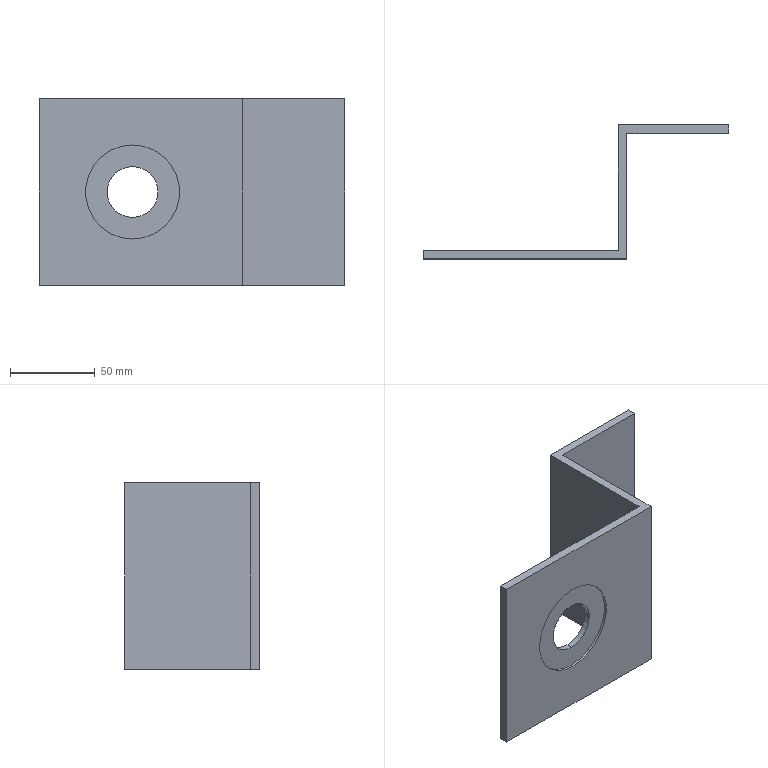Part | STEP file | Guide wheel mechanism revised.sldasm-Part-360 | 1 solid | 15 faces | box 180 x 79 x 110 mm | volume 133597 mm3 | plane 11 | cylinder 4 | commonest cylinder face diameters 30 x2 55.5 x2
STEP:
#1=CARTESIAN_POINT('',(55.,5.,15.));
#2=VERTEX_POINT('',#1);
#3=CARTESIAN_POINT('',(55.,5.,-15.));
#4=VERTEX_POINT('',#3);
#5=CARTESIAN_POINT('',(55.,5.,0.));
#6=DIRECTION('',(0.,-1.,0.));
#7=DIRECTION('',(0.,0.,1.));
#8=AXIS2_PLACEMENT_3D('',#5,#6,#7);
#9=CIRCLE('',#8,15.);
#10=EDGE_CURVE('',#2,#4,#9,.T.);
#11=ORIENTED_EDGE('',*,*,#10,.F.);
#12=CARTESIAN_POINT('',(55.,1.5,15.));
#13=VERTEX_POINT('',#12);
#14=CARTESIAN_POINT('',(55.,79.001,15.));
#15=DIRECTION('',(0.,-1.,0.));
#16=VECTOR('',#15,1000.);
#17=LINE('',#14,#16);
#18=EDGE_CURVE('',#2,#13,#17,.T.);
#19=ORIENTED_EDGE('',*,*,#18,.T.);
#20=CARTESIAN_POINT('',(55.,1.5,-15.));
#21=VERTEX_POINT('',#20);
#22=CARTESIAN_POINT('',(55.,1.5,0.));
#23=DIRECTION('',(0.,-1.,0.));
#24=DIRECTION('',(0.,0.,-1.));
#25=AXIS2_PLACEMENT_3D('',#22,#23,#24);
#26=CIRCLE('',#25,15.);
#27=EDGE_CURVE('',#13,#21,#26,.T.);
#28=ORIENTED_EDGE('',*,*,#27,.T.);
#29=CARTESIAN_POINT('',(55.,79.001,-15.));
#30=DIRECTION('',(0.,-1.,0.));
#31=VECTOR('',#30,1000.);
#32=LINE('',#29,#31);
#33=EDGE_CURVE('',#4,#21,#32,.T.);
#34=ORIENTED_EDGE('',*,*,#33,.F.);
#35=EDGE_LOOP('',(#11,#19,#28,#34));
#36=FACE_OUTER_BOUND('',#35,.T.);
#37=CARTESIAN_POINT('',(55.,79.001,0.));
#38=DIRECTION('',(0.,-1.,0.));
#39=DIRECTION('',(0.,0.,-1.));
#40=AXIS2_PLACEMENT_3D('',#37,#38,#39);
#41=CYLINDRICAL_SURFACE('',#40,15.);
#42=ADVANCED_FACE('',(#36),#41,.F.);
#43=CARTESIAN_POINT('',(55.,1.5,27.75));
#44=VERTEX_POINT('',#43);
#45=CARTESIAN_POINT('',(55.,1.5,-27.75));
#46=VERTEX_POINT('',#45);
#47=CARTESIAN_POINT('',(55.,1.5,0.));
#48=DIRECTION('',(0.,-1.,0.));
#49=DIRECTION('',(0.,0.,-1.));
#50=AXIS2_PLACEMENT_3D('',#47,#48,#49);
#51=CIRCLE('',#50,27.75);
#52=EDGE_CURVE('',#44,#46,#51,.T.);
#53=ORIENTED_EDGE('',*,*,#52,.F.);
#54=CARTESIAN_POINT('',(55.,0.,27.75));
#55=VERTEX_POINT('',#54);
#56=CARTESIAN_POINT('',(55.,1.5,27.75));
#57=DIRECTION('',(0.,-1.,0.));
#58=VECTOR('',#57,1000.);
#59=LINE('',#56,#58);
#60=EDGE_CURVE('',#44,#55,#59,.T.);
#61=ORIENTED_EDGE('',*,*,#60,.T.);
#62=CARTESIAN_POINT('',(55.,0.,-27.75));
#63=VERTEX_POINT('',#62);
#64=CARTESIAN_POINT('',(55.,0.,0.));
#65=DIRECTION('',(0.,-1.,0.));
#66=DIRECTION('',(0.,0.,-1.));
#67=AXIS2_PLACEMENT_3D('',#64,#65,#66);
#68=CIRCLE('',#67,27.75);
#69=EDGE_CURVE('',#55,#63,#68,.T.);
#70=ORIENTED_EDGE('',*,*,#69,.T.);
#71=CARTESIAN_POINT('',(55.,1.5,-27.75));
#72=DIRECTION('',(0.,-1.,0.));
#73=VECTOR('',#72,1000.);
#74=LINE('',#71,#73);
#75=EDGE_CURVE('',#46,#63,#74,.T.);
#76=ORIENTED_EDGE('',*,*,#75,.F.);
#77=EDGE_LOOP('',(#53,#61,#70,#76));
#78=FACE_OUTER_BOUND('',#77,.T.);
#79=CARTESIAN_POINT('',(55.,1.5,0.));
#80=DIRECTION('',(0.,-1.,0.));
#81=DIRECTION('',(0.,0.,-1.));
#82=AXIS2_PLACEMENT_3D('',#79,#80,#81);
#83=CYLINDRICAL_SURFACE('',#82,27.75);
#84=ADVANCED_FACE('',(#78),#83,.F.);
#85=CARTESIAN_POINT('',(120.,74.,-55.));
#86=VERTEX_POINT('',#85);
#87=CARTESIAN_POINT('',(180.,74.,-55.));
#88=VERTEX_POINT('',#87);
#89=CARTESIAN_POINT('',(120.,74.,-55.));
#90=DIRECTION('',(1.,0.,0.));
#91=VECTOR('',#90,1000.);
#92=LINE('',#89,#91);
#93=EDGE_CURVE('',#86,#88,#92,.T.);
#94=ORIENTED_EDGE('',*,*,#93,.T.);
#95=CARTESIAN_POINT('',(180.,74.,55.));
#96=VERTEX_POINT('',#95);
#97=CARTESIAN_POINT('',(180.,74.,55.));
#98=DIRECTION('',(0.,0.,-1.));
#99=VECTOR('',#98,1000.);
#100=LINE('',#97,#99);
#101=EDGE_CURVE('',#96,#88,#100,.T.);
#102=ORIENTED_EDGE('',*,*,#101,.F.);
#103=CARTESIAN_POINT('',(120.,74.,55.));
#104=VERTEX_POINT('',#103);
#105=CARTESIAN_POINT('',(120.,74.,55.));
#106=DIRECTION('',(1.,0.,0.));
#107=VECTOR('',#106,1000.);
#108=LINE('',#105,#107);
#109=EDGE_CURVE('',#104,#96,#108,.T.);
#110=ORIENTED_EDGE('',*,*,#109,.F.);
#111=CARTESIAN_POINT('',(120.,74.,55.));
#112=DIRECTION('',(0.,0.,-1.));
#113=VECTOR('',#112,1000.);
#114=LINE('',#111,#113);
#115=EDGE_CURVE('',#104,#86,#114,.T.);
#116=ORIENTED_EDGE('',*,*,#115,.T.);
#117=EDGE_LOOP('',(#94,#102,#110,#116));
#118=FACE_OUTER_BOUND('',#117,.T.);
#119=CARTESIAN_POINT('',(120.,74.,55.));
#120=DIRECTION('',(0.,1.,0.));
#121=DIRECTION('',(0.,0.,1.));
#122=AXIS2_PLACEMENT_3D('',#119,#120,#121);
#123=PLANE('',#122);
#124=ADVANCED_FACE('',(#118),#123,.F.);
#125=CARTESIAN_POINT('',(180.,79.,-55.));
#126=VERTEX_POINT('',#125);
#127=CARTESIAN_POINT('',(180.,79.,-55.));
#128=DIRECTION('',(0.,-1.,0.));
#129=VECTOR('',#128,1000.);
#130=LINE('',#127,#129);
#131=EDGE_CURVE('',#126,#88,#130,.T.);
#132=ORIENTED_EDGE('',*,*,#131,.F.);
#133=CARTESIAN_POINT('',(180.,79.,55.));
#134=VERTEX_POINT('',#133);
#135=CARTESIAN_POINT('',(180.,79.,55.));
#136=DIRECTION('',(0.,0.,-1.));
#137=VECTOR('',#136,1000.);
#138=LINE('',#135,#137);
#139=EDGE_CURVE('',#134,#126,#138,.T.);
#140=ORIENTED_EDGE('',*,*,#139,.F.);
#141=CARTESIAN_POINT('',(180.,79.,55.));
#142=DIRECTION('',(0.,-1.,0.));
#143=VECTOR('',#142,1000.);
#144=LINE('',#141,#143);
#145=EDGE_CURVE('',#134,#96,#144,.T.);
#146=ORIENTED_EDGE('',*,*,#145,.T.);
#147=ORIENTED_EDGE('',*,*,#101,.T.);
#148=EDGE_LOOP('',(#132,#140,#146,#147));
#149=FACE_OUTER_BOUND('',#148,.T.);
#150=CARTESIAN_POINT('',(180.,79.,55.));
#151=DIRECTION('',(1.,0.,0.));
#152=DIRECTION('',(0.,0.,-1.));
#153=AXIS2_PLACEMENT_3D('',#150,#151,#152);
#154=PLANE('',#153);
#155=ADVANCED_FACE('',(#149),#154,.T.);
#156=CARTESIAN_POINT('',(115.,79.,-55.));
#157=VERTEX_POINT('',#156);
#158=CARTESIAN_POINT('',(120.,79.,-55.));
#159=DIRECTION('',(1.,0.,0.));
#160=VECTOR('',#159,1000.);
#161=LINE('',#158,#160);
#162=EDGE_CURVE('',#157,#126,#161,.T.);
#163=ORIENTED_EDGE('',*,*,#162,.F.);
#164=CARTESIAN_POINT('',(115.,79.,55.));
#165=VERTEX_POINT('',#164);
#166=CARTESIAN_POINT('',(115.,79.,55.));
#167=DIRECTION('',(0.,0.,-1.));
#168=VECTOR('',#167,1000.);
#169=LINE('',#166,#168);
#170=EDGE_CURVE('',#165,#157,#169,.T.);
#171=ORIENTED_EDGE('',*,*,#170,.F.);
#172=CARTESIAN_POINT('',(120.,79.,55.));
#173=DIRECTION('',(1.,0.,0.));
#174=VECTOR('',#173,1000.);
#175=LINE('',#172,#174);
#176=EDGE_CURVE('',#165,#134,#175,.T.);
#177=ORIENTED_EDGE('',*,*,#176,.T.);
#178=ORIENTED_EDGE('',*,*,#139,.T.);
#179=EDGE_LOOP('',(#163,#171,#177,#178));
#180=FACE_OUTER_BOUND('',#179,.T.);
#181=CARTESIAN_POINT('',(120.,79.,55.));
#182=DIRECTION('',(0.,1.,0.));
#183=DIRECTION('',(0.,0.,1.));
#184=AXIS2_PLACEMENT_3D('',#181,#182,#183);
#185=PLANE('',#184);
#186=ADVANCED_FACE('',(#180),#185,.T.);
#187=CARTESIAN_POINT('',(115.,5.,-55.));
#188=VERTEX_POINT('',#187);
#189=CARTESIAN_POINT('',(115.,0.,-55.));
#190=DIRECTION('',(0.,1.,0.));
#191=VECTOR('',#190,1000.);
#192=LINE('',#189,#191);
#193=EDGE_CURVE('',#188,#157,#192,.T.);
#194=ORIENTED_EDGE('',*,*,#193,.F.);
#195=CARTESIAN_POINT('',(115.,5.,55.));
#196=VERTEX_POINT('',#195);
#197=CARTESIAN_POINT('',(115.,5.,55.));
#198=DIRECTION('',(0.,0.,-1.));
#199=VECTOR('',#198,1000.);
#200=LINE('',#197,#199);
#201=EDGE_CURVE('',#196,#188,#200,.T.);
#202=ORIENTED_EDGE('',*,*,#201,.F.);
#203=CARTESIAN_POINT('',(115.,0.,55.));
#204=DIRECTION('',(0.,1.,0.));
#205=VECTOR('',#204,1000.);
#206=LINE('',#203,#205);
#207=EDGE_CURVE('',#196,#165,#206,.T.);
#208=ORIENTED_EDGE('',*,*,#207,.T.);
#209=ORIENTED_EDGE('',*,*,#170,.T.);
#210=EDGE_LOOP('',(#194,#202,#208,#209));
#211=FACE_OUTER_BOUND('',#210,.T.);
#212=CARTESIAN_POINT('',(115.,0.,55.));
#213=DIRECTION('',(-1.,0.,0.));
#214=DIRECTION('',(0.,0.,1.));
#215=AXIS2_PLACEMENT_3D('',#212,#213,#214);
#216=PLANE('',#215);
#217=ADVANCED_FACE('',(#211),#216,.T.);
#218=CARTESIAN_POINT('',(55.,5.,0.));
#219=DIRECTION('',(0.,-1.,0.));
#220=DIRECTION('',(0.,0.,1.));
#221=AXIS2_PLACEMENT_3D('',#218,#219,#220);
#222=CIRCLE('',#221,15.);
#223=EDGE_CURVE('',#4,#2,#222,.T.);
#224=ORIENTED_EDGE('',*,*,#223,.T.);
#225=ORIENTED_EDGE('',*,*,#10,.T.);
#226=EDGE_LOOP('',(#224,#225));
#227=FACE_BOUND('',#226,.T.);
#228=CARTESIAN_POINT('',(0.,5.,-55.));
#229=VERTEX_POINT('',#228);
#230=CARTESIAN_POINT('',(0.,5.,-55.));
#231=DIRECTION('',(1.,0.,0.));
#232=VECTOR('',#231,1000.);
#233=LINE('',#230,#232);
#234=EDGE_CURVE('',#229,#188,#233,.T.);
#235=ORIENTED_EDGE('',*,*,#234,.F.);
#236=CARTESIAN_POINT('',(0.,5.,55.));
#237=VERTEX_POINT('',#236);
#238=CARTESIAN_POINT('',(0.,5.,55.));
#239=DIRECTION('',(0.,0.,-1.));
#240=VECTOR('',#239,1000.);
#241=LINE('',#238,#240);
#242=EDGE_CURVE('',#237,#229,#241,.T.);
#243=ORIENTED_EDGE('',*,*,#242,.F.);
#244=CARTESIAN_POINT('',(0.,5.,55.));
#245=DIRECTION('',(1.,0.,0.));
#246=VECTOR('',#245,1000.);
#247=LINE('',#244,#246);
#248=EDGE_CURVE('',#237,#196,#247,.T.);
#249=ORIENTED_EDGE('',*,*,#248,.T.);
#250=ORIENTED_EDGE('',*,*,#201,.T.);
#251=EDGE_LOOP('',(#235,#243,#249,#250));
#252=FACE_OUTER_BOUND('',#251,.T.);
#253=CARTESIAN_POINT('',(0.,5.,55.));
#254=DIRECTION('',(0.,1.,0.));
#255=DIRECTION('',(0.,0.,1.));
#256=AXIS2_PLACEMENT_3D('',#253,#254,#255);
#257=PLANE('',#256);
#258=ADVANCED_FACE('',(#227,#252),#257,.T.);
#259=CARTESIAN_POINT('',(0.,0.,-55.));
#260=VERTEX_POINT('',#259);
#261=CARTESIAN_POINT('',(0.,0.,-55.));
#262=DIRECTION('',(0.,1.,0.));
#263=VECTOR('',#262,1000.);
#264=LINE('',#261,#263);
#265=EDGE_CURVE('',#260,#229,#264,.T.);
#266=ORIENTED_EDGE('',*,*,#265,.F.);
#267=CARTESIAN_POINT('',(0.,0.,55.));
#268=VERTEX_POINT('',#267);
#269=CARTESIAN_POINT('',(0.,0.,55.));
#270=DIRECTION('',(0.,0.,-1.));
#271=VECTOR('',#270,1000.);
#272=LINE('',#269,#271);
#273=EDGE_CURVE('',#268,#260,#272,.T.);
#274=ORIENTED_EDGE('',*,*,#273,.F.);
#275=CARTESIAN_POINT('',(0.,0.,55.));
#276=DIRECTION('',(0.,1.,0.));
#277=VECTOR('',#276,1000.);
#278=LINE('',#275,#277);
#279=EDGE_CURVE('',#268,#237,#278,.T.);
#280=ORIENTED_EDGE('',*,*,#279,.T.);
#281=ORIENTED_EDGE('',*,*,#242,.T.);
#282=EDGE_LOOP('',(#266,#274,#280,#281));
#283=FACE_OUTER_BOUND('',#282,.T.);
#284=CARTESIAN_POINT('',(0.,0.,55.));
#285=DIRECTION('',(-1.,0.,0.));
#286=DIRECTION('',(0.,0.,1.));
#287=AXIS2_PLACEMENT_3D('',#284,#285,#286);
#288=PLANE('',#287);
#289=ADVANCED_FACE('',(#283),#288,.T.);
#290=CARTESIAN_POINT('',(55.,0.,0.));
#291=DIRECTION('',(0.,-1.,0.));
#292=DIRECTION('',(0.,0.,-1.));
#293=AXIS2_PLACEMENT_3D('',#290,#291,#292);
#294=CIRCLE('',#293,27.75);
#295=EDGE_CURVE('',#63,#55,#294,.T.);
#296=ORIENTED_EDGE('',*,*,#295,.F.);
#297=ORIENTED_EDGE('',*,*,#69,.F.);
#298=EDGE_LOOP('',(#296,#297));
#299=FACE_BOUND('',#298,.T.);
#300=CARTESIAN_POINT('',(120.,0.,-55.));
#301=VERTEX_POINT('',#300);
#302=CARTESIAN_POINT('',(0.,0.,-55.));
#303=DIRECTION('',(1.,0.,0.));
#304=VECTOR('',#303,1000.);
#305=LINE('',#302,#304);
#306=EDGE_CURVE('',#260,#301,#305,.T.);
#307=ORIENTED_EDGE('',*,*,#306,.T.);
#308=CARTESIAN_POINT('',(120.,0.,55.));
#309=VERTEX_POINT('',#308);
#310=CARTESIAN_POINT('',(120.,0.,55.));
#311=DIRECTION('',(0.,0.,-1.));
#312=VECTOR('',#311,1000.);
#313=LINE('',#310,#312);
#314=EDGE_CURVE('',#309,#301,#313,.T.);
#315=ORIENTED_EDGE('',*,*,#314,.F.);
#316=CARTESIAN_POINT('',(0.,0.,55.));
#317=DIRECTION('',(1.,0.,0.));
#318=VECTOR('',#317,1000.);
#319=LINE('',#316,#318);
#320=EDGE_CURVE('',#268,#309,#319,.T.);
#321=ORIENTED_EDGE('',*,*,#320,.F.);
#322=ORIENTED_EDGE('',*,*,#273,.T.);
#323=EDGE_LOOP('',(#307,#315,#321,#322));
#324=FACE_OUTER_BOUND('',#323,.T.);
#325=CARTESIAN_POINT('',(0.,0.,55.));
#326=DIRECTION('',(0.,1.,0.));
#327=DIRECTION('',(0.,0.,1.));
#328=AXIS2_PLACEMENT_3D('',#325,#326,#327);
#329=PLANE('',#328);
#330=ADVANCED_FACE('',(#299,#324),#329,.F.);
#331=CARTESIAN_POINT('',(120.,0.,-55.));
#332=DIRECTION('',(0.,1.,0.));
#333=VECTOR('',#332,1000.);
#334=LINE('',#331,#333);
#335=EDGE_CURVE('',#301,#86,#334,.T.);
#336=ORIENTED_EDGE('',*,*,#335,.T.);
#337=ORIENTED_EDGE('',*,*,#115,.F.);
#338=CARTESIAN_POINT('',(120.,0.,55.));
#339=DIRECTION('',(0.,1.,0.));
#340=VECTOR('',#339,1000.);
#341=LINE('',#338,#340);
#342=EDGE_CURVE('',#309,#104,#341,.T.);
#343=ORIENTED_EDGE('',*,*,#342,.F.);
#344=ORIENTED_EDGE('',*,*,#314,.T.);
#345=EDGE_LOOP('',(#336,#337,#343,#344));
#346=FACE_OUTER_BOUND('',#345,.T.);
#347=CARTESIAN_POINT('',(120.,0.,55.));
#348=DIRECTION('',(-1.,0.,0.));
#349=DIRECTION('',(0.,0.,1.));
#350=AXIS2_PLACEMENT_3D('',#347,#348,#349);
#351=PLANE('',#350);
#352=ADVANCED_FACE('',(#346),#351,.F.);
#353=ORIENTED_EDGE('',*,*,#109,.T.);
#354=ORIENTED_EDGE('',*,*,#145,.F.);
#355=ORIENTED_EDGE('',*,*,#176,.F.);
#356=ORIENTED_EDGE('',*,*,#207,.F.);
#357=ORIENTED_EDGE('',*,*,#248,.F.);
#358=ORIENTED_EDGE('',*,*,#279,.F.);
#359=ORIENTED_EDGE('',*,*,#320,.T.);
#360=ORIENTED_EDGE('',*,*,#342,.T.);
#361=EDGE_LOOP('',(#353,#354,#355,#356,#357,#358,#359,#360));
#362=FACE_OUTER_BOUND('',#361,.T.);
#363=CARTESIAN_POINT('',(0.,0.,55.));
#364=DIRECTION('',(0.,0.,-1.));
#365=DIRECTION('',(-1.,0.,0.));
#366=AXIS2_PLACEMENT_3D('',#363,#364,#365);
#367=PLANE('',#366);
#368=ADVANCED_FACE('',(#362),#367,.F.);
#369=ORIENTED_EDGE('',*,*,#93,.F.);
#370=ORIENTED_EDGE('',*,*,#335,.F.);
#371=ORIENTED_EDGE('',*,*,#306,.F.);
#372=ORIENTED_EDGE('',*,*,#265,.T.);
#373=ORIENTED_EDGE('',*,*,#234,.T.);
#374=ORIENTED_EDGE('',*,*,#193,.T.);
#375=ORIENTED_EDGE('',*,*,#162,.T.);
#376=ORIENTED_EDGE('',*,*,#131,.T.);
#377=EDGE_LOOP('',(#369,#370,#371,#372,#373,#374,#375,#376));
#378=FACE_OUTER_BOUND('',#377,.T.);
#379=CARTESIAN_POINT('',(0.,0.,-55.));
#380=DIRECTION('',(0.,0.,-1.));
#381=DIRECTION('',(-1.,0.,0.));
#382=AXIS2_PLACEMENT_3D('',#379,#380,#381);
#383=PLANE('',#382);
#384=ADVANCED_FACE('',(#378),#383,.T.);
#385=ORIENTED_EDGE('',*,*,#60,.F.);
#386=CARTESIAN_POINT('',(55.,1.5,0.));
#387=DIRECTION('',(0.,-1.,0.));
#388=DIRECTION('',(0.,0.,-1.));
#389=AXIS2_PLACEMENT_3D('',#386,#387,#388);
#390=CIRCLE('',#389,27.75);
#391=EDGE_CURVE('',#46,#44,#390,.T.);
#392=ORIENTED_EDGE('',*,*,#391,.F.);
#393=ORIENTED_EDGE('',*,*,#75,.T.);
#394=ORIENTED_EDGE('',*,*,#295,.T.);
#395=EDGE_LOOP('',(#385,#392,#393,#394));
#396=FACE_OUTER_BOUND('',#395,.T.);
#397=CARTESIAN_POINT('',(55.,1.5,0.));
#398=DIRECTION('',(0.,-1.,0.));
#399=DIRECTION('',(0.,0.,-1.));
#400=AXIS2_PLACEMENT_3D('',#397,#398,#399);
#401=CYLINDRICAL_SURFACE('',#400,27.75);
#402=ADVANCED_FACE('',(#396),#401,.F.);
#403=CARTESIAN_POINT('',(55.,1.5,0.));
#404=DIRECTION('',(0.,-1.,0.));
#405=DIRECTION('',(0.,0.,-1.));
#406=AXIS2_PLACEMENT_3D('',#403,#404,#405);
#407=CIRCLE('',#406,15.);
#408=EDGE_CURVE('',#21,#13,#407,.T.);
#409=ORIENTED_EDGE('',*,*,#408,.F.);
#410=ORIENTED_EDGE('',*,*,#27,.F.);
#411=EDGE_LOOP('',(#409,#410));
#412=FACE_BOUND('',#411,.T.);
#413=ORIENTED_EDGE('',*,*,#391,.T.);
#414=ORIENTED_EDGE('',*,*,#52,.T.);
#415=EDGE_LOOP('',(#413,#414));
#416=FACE_OUTER_BOUND('',#415,.T.);
#417=CARTESIAN_POINT('',(55.,1.5,0.));
#418=DIRECTION('',(0.,-1.,0.));
#419=DIRECTION('',(0.,0.,-1.));
#420=AXIS2_PLACEMENT_3D('',#417,#418,#419);
#421=PLANE('',#420);
#422=ADVANCED_FACE('',(#412,#416),#421,.T.);
#423=ORIENTED_EDGE('',*,*,#18,.F.);
#424=ORIENTED_EDGE('',*,*,#223,.F.);
#425=ORIENTED_EDGE('',*,*,#33,.T.);
#426=ORIENTED_EDGE('',*,*,#408,.T.);
#427=EDGE_LOOP('',(#423,#424,#425,#426));
#428=FACE_OUTER_BOUND('',#427,.T.);
#429=CARTESIAN_POINT('',(55.,79.001,0.));
#430=DIRECTION('',(0.,-1.,0.));
#431=DIRECTION('',(0.,0.,-1.));
#432=AXIS2_PLACEMENT_3D('',#429,#430,#431);
#433=CYLINDRICAL_SURFACE('',#432,15.);
#434=ADVANCED_FACE('',(#428),#433,.F.);
#435=CLOSED_SHELL('',(#42,#84,#124,#155,#186,#217,#258,#289,#330,#352,#368,#384,#402,#422,#434));
#436=MANIFOLD_SOLID_BREP('',#435);
#437=CARTESIAN_POINT('',(0.,0.,0.));
#438=DIRECTION('',(0.,0.,1.));
#439=DIRECTION('',(1.,0.,0.));
#440=AXIS2_PLACEMENT_3D('',#437,#438,#439);
#441=(LENGTH_UNIT()NAMED_UNIT(*)SI_UNIT(.MILLI.,.METRE.));
#442=UNCERTAINTY_MEASURE_WITH_UNIT(LENGTH_MEASURE(0.00001),#441,'','');
#443=(NAMED_UNIT(*)PLANE_ANGLE_UNIT()SI_UNIT($,.RADIAN.));
#444=(NAMED_UNIT(*)SI_UNIT($,.STERADIAN.)SOLID_ANGLE_UNIT());
#445=(GEOMETRIC_REPRESENTATION_CONTEXT(3)GLOBAL_UNCERTAINTY_ASSIGNED_CONTEXT((#442))GLOBAL_UNIT_ASSIGNED_CONTEXT((#441,#443,#444))REPRESENTATION_CONTEXT('',''));
#446=ADVANCED_BREP_SHAPE_REPRESENTATION('',(#436,#440),#445);